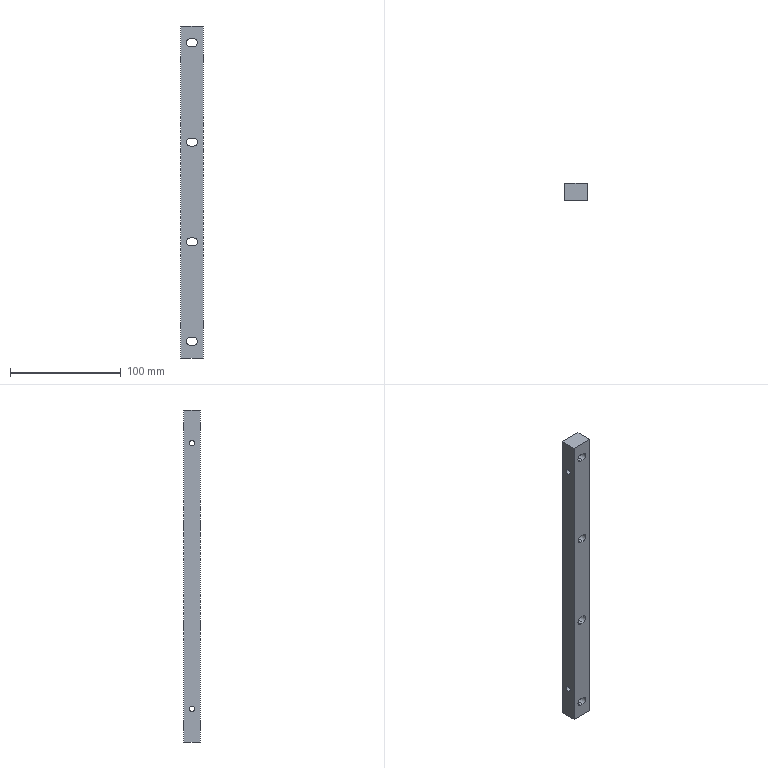Part | NX | 1 solid | 34 faces | box 20 x 15 x 300 mm | volume 85636 mm3 | cylinder 16 | plane 14 | cone 4 | commonest cylinder face diameters 7 x12 5 x4
STEP:
#1=CARTESIAN_POINT('',(263.6,-113.5,-473.5));
#2=VERTEX_POINT('',#1);
#3=CARTESIAN_POINT('',(283.6,-113.5,-473.5));
#4=VERTEX_POINT('',#3);
#5=CARTESIAN_POINT('',(237.204,-113.5,-473.5));
#6=DIRECTION('',(1.,0.,0.));
#7=VECTOR('',#6,1000.);
#8=LINE('',#5,#7);
#9=EDGE_CURVE('',#2,#4,#8,.T.);
#10=ORIENTED_EDGE('',*,*,#9,.F.);
#11=CARTESIAN_POINT('',(263.6,-98.5,-473.5));
#12=VERTEX_POINT('',#11);
#13=CARTESIAN_POINT('',(263.6,-112.5,-473.5));
#14=DIRECTION('',(0.,1.,0.));
#15=VECTOR('',#14,1000.);
#16=LINE('',#13,#15);
#17=EDGE_CURVE('',#2,#12,#16,.T.);
#18=ORIENTED_EDGE('',*,*,#17,.T.);
#19=CARTESIAN_POINT('',(283.6,-98.5,-473.5));
#20=VERTEX_POINT('',#19);
#21=CARTESIAN_POINT('',(237.204,-98.5,-473.5));
#22=DIRECTION('',(-1.,0.,0.));
#23=VECTOR('',#22,1000.);
#24=LINE('',#21,#23);
#25=EDGE_CURVE('',#20,#12,#24,.T.);
#26=ORIENTED_EDGE('',*,*,#25,.F.);
#27=CARTESIAN_POINT('',(283.6,-112.5,-473.5));
#28=DIRECTION('',(0.,-1.,0.));
#29=VECTOR('',#28,1000.);
#30=LINE('',#27,#29);
#31=EDGE_CURVE('',#20,#4,#30,.T.);
#32=ORIENTED_EDGE('',*,*,#31,.T.);
#33=EDGE_LOOP('',(#10,#18,#26,#32));
#34=FACE_BOUND('',#33,.T.);
#35=CARTESIAN_POINT('',(263.6,-112.5,-473.5));
#36=DIRECTION('',(0.,0.,-1.));
#37=DIRECTION('',(0.,-1.,0.));
#38=AXIS2_PLACEMENT_3D('',#35,#36,#37);
#39=PLANE('',#38);
#40=ADVANCED_FACE('',(#34),#39,.T.);
#41=CARTESIAN_POINT('',(263.6,-113.5,-173.5));
#42=VERTEX_POINT('',#41);
#43=CARTESIAN_POINT('',(263.6,-113.5,-531.056));
#44=DIRECTION('',(0.,0.,1.));
#45=VECTOR('',#44,1000.);
#46=LINE('',#43,#45);
#47=EDGE_CURVE('',#2,#42,#46,.T.);
#48=ORIENTED_EDGE('',*,*,#47,.T.);
#49=CARTESIAN_POINT('',(263.6,-98.5,-173.5));
#50=VERTEX_POINT('',#49);
#51=CARTESIAN_POINT('',(263.6,-112.5,-173.5));
#52=DIRECTION('',(0.,-1.,0.));
#53=VECTOR('',#52,1000.);
#54=LINE('',#51,#53);
#55=EDGE_CURVE('',#50,#42,#54,.T.);
#56=ORIENTED_EDGE('',*,*,#55,.F.);
#57=CARTESIAN_POINT('',(263.6,-98.5,-531.056));
#58=DIRECTION('',(0.,0.,1.));
#59=VECTOR('',#58,1000.);
#60=LINE('',#57,#59);
#61=EDGE_CURVE('',#12,#50,#60,.T.);
#62=ORIENTED_EDGE('',*,*,#61,.F.);
#63=ORIENTED_EDGE('',*,*,#17,.F.);
#64=EDGE_LOOP('',(#48,#56,#62,#63));
#65=FACE_BOUND('',#64,.T.);
#66=CARTESIAN_POINT('',(263.6,-106.,-201.));
#67=VERTEX_POINT('',#66);
#68=CARTESIAN_POINT('',(263.6,-106.,-206.));
#69=VERTEX_POINT('',#68);
#70=CARTESIAN_POINT('',(263.6,-106.,-203.5));
#71=DIRECTION('',(1.,0.,0.));
#72=DIRECTION('',(0.,0.,1.));
#73=AXIS2_PLACEMENT_3D('',#70,#71,#72);
#74=CIRCLE('',#73,2.5);
#75=EDGE_CURVE('',#67,#69,#74,.T.);
#76=ORIENTED_EDGE('',*,*,#75,.T.);
#77=CARTESIAN_POINT('',(263.6,-106.,-203.5));
#78=DIRECTION('',(1.,0.,0.));
#79=DIRECTION('',(0.,0.,1.));
#80=AXIS2_PLACEMENT_3D('',#77,#78,#79);
#81=CIRCLE('',#80,2.5);
#82=EDGE_CURVE('',#69,#67,#81,.T.);
#83=ORIENTED_EDGE('',*,*,#82,.T.);
#84=EDGE_LOOP('',(#76,#83));
#85=FACE_BOUND('',#84,.T.);
#86=CARTESIAN_POINT('',(263.6,-106.,-446.));
#87=VERTEX_POINT('',#86);
#88=CARTESIAN_POINT('',(263.6,-106.,-441.));
#89=VERTEX_POINT('',#88);
#90=CARTESIAN_POINT('',(263.6,-106.,-443.5));
#91=DIRECTION('',(1.,0.,0.));
#92=DIRECTION('',(0.,0.,1.));
#93=AXIS2_PLACEMENT_3D('',#90,#91,#92);
#94=CIRCLE('',#93,2.5);
#95=EDGE_CURVE('',#87,#89,#94,.T.);
#96=ORIENTED_EDGE('',*,*,#95,.T.);
#97=CARTESIAN_POINT('',(263.6,-106.,-443.5));
#98=DIRECTION('',(1.,0.,0.));
#99=DIRECTION('',(0.,0.,1.));
#100=AXIS2_PLACEMENT_3D('',#97,#98,#99);
#101=CIRCLE('',#100,2.5);
#102=EDGE_CURVE('',#89,#87,#101,.T.);
#103=ORIENTED_EDGE('',*,*,#102,.T.);
#104=EDGE_LOOP('',(#96,#103));
#105=FACE_BOUND('',#104,.T.);
#106=CARTESIAN_POINT('',(263.6,-112.5,-173.5));
#107=DIRECTION('',(-1.,0.,0.));
#108=DIRECTION('',(0.,0.,1.));
#109=AXIS2_PLACEMENT_3D('',#106,#107,#108);
#110=PLANE('',#109);
#111=ADVANCED_FACE('',(#65,#85,#105),#110,.T.);
#112=CARTESIAN_POINT('',(283.6,-113.5,-173.5));
#113=VERTEX_POINT('',#112);
#114=CARTESIAN_POINT('',(237.204,-113.5,-173.5));
#115=DIRECTION('',(-1.,0.,0.));
#116=VECTOR('',#115,1000.);
#117=LINE('',#114,#116);
#118=EDGE_CURVE('',#113,#42,#117,.T.);
#119=ORIENTED_EDGE('',*,*,#118,.F.);
#120=CARTESIAN_POINT('',(283.6,-98.5,-173.5));
#121=VERTEX_POINT('',#120);
#122=CARTESIAN_POINT('',(283.6,-112.5,-173.5));
#123=DIRECTION('',(0.,1.,0.));
#124=VECTOR('',#123,1000.);
#125=LINE('',#122,#124);
#126=EDGE_CURVE('',#113,#121,#125,.T.);
#127=ORIENTED_EDGE('',*,*,#126,.T.);
#128=CARTESIAN_POINT('',(237.204,-98.5,-173.5));
#129=DIRECTION('',(1.,0.,0.));
#130=VECTOR('',#129,1000.);
#131=LINE('',#128,#130);
#132=EDGE_CURVE('',#50,#121,#131,.T.);
#133=ORIENTED_EDGE('',*,*,#132,.F.);
#134=ORIENTED_EDGE('',*,*,#55,.T.);
#135=EDGE_LOOP('',(#119,#127,#133,#134));
#136=FACE_BOUND('',#135,.T.);
#137=CARTESIAN_POINT('',(278.6,-112.5,-173.5));
#138=DIRECTION('',(0.,0.,1.));
#139=DIRECTION('',(1.,0.,0.));
#140=AXIS2_PLACEMENT_3D('',#137,#138,#139);
#141=PLANE('',#140);
#142=ADVANCED_FACE('',(#136),#141,.T.);
#143=CARTESIAN_POINT('',(283.6,-113.5,-531.056));
#144=DIRECTION('',(0.,0.,-1.));
#145=VECTOR('',#144,1000.);
#146=LINE('',#143,#145);
#147=EDGE_CURVE('',#113,#4,#146,.T.);
#148=ORIENTED_EDGE('',*,*,#147,.T.);
#149=ORIENTED_EDGE('',*,*,#31,.F.);
#150=CARTESIAN_POINT('',(283.6,-98.5,-531.056));
#151=DIRECTION('',(0.,0.,-1.));
#152=VECTOR('',#151,1000.);
#153=LINE('',#150,#152);
#154=EDGE_CURVE('',#121,#20,#153,.T.);
#155=ORIENTED_EDGE('',*,*,#154,.F.);
#156=ORIENTED_EDGE('',*,*,#126,.F.);
#157=EDGE_LOOP('',(#148,#149,#155,#156));
#158=FACE_BOUND('',#157,.T.);
#159=CARTESIAN_POINT('',(283.6,-109.45,-203.5));
#160=VERTEX_POINT('',#159);
#161=CARTESIAN_POINT('',(283.6,-102.55,-203.5));
#162=VERTEX_POINT('',#161);
#163=CARTESIAN_POINT('',(283.6,-106.,-203.5));
#164=DIRECTION('',(1.,0.,0.));
#165=DIRECTION('',(0.,0.,1.));
#166=AXIS2_PLACEMENT_3D('',#163,#164,#165);
#167=CIRCLE('',#166,3.45);
#168=EDGE_CURVE('',#160,#162,#167,.T.);
#169=ORIENTED_EDGE('',*,*,#168,.F.);
#170=CARTESIAN_POINT('',(283.6,-106.,-203.5));
#171=DIRECTION('',(1.,0.,0.));
#172=DIRECTION('',(0.,0.,1.));
#173=AXIS2_PLACEMENT_3D('',#170,#171,#172);
#174=CIRCLE('',#173,3.45);
#175=EDGE_CURVE('',#162,#160,#174,.T.);
#176=ORIENTED_EDGE('',*,*,#175,.F.);
#177=EDGE_LOOP('',(#169,#176));
#178=FACE_BOUND('',#177,.T.);
#179=CARTESIAN_POINT('',(283.6,-109.45,-443.5));
#180=VERTEX_POINT('',#179);
#181=CARTESIAN_POINT('',(283.6,-102.55,-443.5));
#182=VERTEX_POINT('',#181);
#183=CARTESIAN_POINT('',(283.6,-106.,-443.5));
#184=DIRECTION('',(1.,0.,0.));
#185=DIRECTION('',(0.,0.,1.));
#186=AXIS2_PLACEMENT_3D('',#183,#184,#185);
#187=CIRCLE('',#186,3.45);
#188=EDGE_CURVE('',#180,#182,#187,.T.);
#189=ORIENTED_EDGE('',*,*,#188,.F.);
#190=CARTESIAN_POINT('',(283.6,-106.,-443.5));
#191=DIRECTION('',(1.,0.,0.));
#192=DIRECTION('',(0.,0.,1.));
#193=AXIS2_PLACEMENT_3D('',#190,#191,#192);
#194=CIRCLE('',#193,3.45);
#195=EDGE_CURVE('',#182,#180,#194,.T.);
#196=ORIENTED_EDGE('',*,*,#195,.F.);
#197=EDGE_LOOP('',(#189,#196));
#198=FACE_BOUND('',#197,.T.);
#199=CARTESIAN_POINT('',(283.6,-112.5,-473.5));
#200=DIRECTION('',(1.,0.,0.));
#201=DIRECTION('',(0.,1.,0.));
#202=AXIS2_PLACEMENT_3D('',#199,#200,#201);
#203=PLANE('',#202);
#204=ADVANCED_FACE('',(#158,#178,#198),#203,.T.);
#205=CARTESIAN_POINT('',(283.052,-108.5,-203.5));
#206=VERTEX_POINT('',#205);
#207=CARTESIAN_POINT('',(283.052,-106.,-206.));
#208=VERTEX_POINT('',#207);
#209=CARTESIAN_POINT('',(283.052,-106.,-203.5));
#210=DIRECTION('',(1.,0.,0.));
#211=DIRECTION('',(0.,0.,1.));
#212=AXIS2_PLACEMENT_3D('',#209,#210,#211);
#213=CIRCLE('',#212,2.5);
#214=EDGE_CURVE('',#206,#208,#213,.T.);
#215=ORIENTED_EDGE('',*,*,#214,.T.);
#216=CARTESIAN_POINT('',(283.6,-106.,-206.));
#217=DIRECTION('',(1.,0.,0.));
#218=VECTOR('',#217,1000.);
#219=LINE('',#216,#218);
#220=EDGE_CURVE('',#208,#69,#219,.F.);
#221=ORIENTED_EDGE('',*,*,#220,.T.);
#222=ORIENTED_EDGE('',*,*,#75,.F.);
#223=CARTESIAN_POINT('',(283.052,-106.,-201.));
#224=VERTEX_POINT('',#223);
#225=CARTESIAN_POINT('',(283.6,-106.,-201.));
#226=DIRECTION('',(1.,0.,0.));
#227=VECTOR('',#226,1000.);
#228=LINE('',#225,#227);
#229=EDGE_CURVE('',#224,#67,#228,.F.);
#230=ORIENTED_EDGE('',*,*,#229,.F.);
#231=CARTESIAN_POINT('',(283.052,-106.,-203.5));
#232=DIRECTION('',(1.,0.,0.));
#233=DIRECTION('',(0.,0.,1.));
#234=AXIS2_PLACEMENT_3D('',#231,#232,#233);
#235=CIRCLE('',#234,2.5);
#236=EDGE_CURVE('',#224,#206,#235,.T.);
#237=ORIENTED_EDGE('',*,*,#236,.T.);
#238=EDGE_LOOP('',(#215,#221,#222,#230,#237));
#239=FACE_BOUND('',#238,.T.);
#240=CARTESIAN_POINT('',(283.6,-106.,-203.5));
#241=DIRECTION('',(1.,0.,0.));
#242=DIRECTION('',(0.,0.,1.));
#243=AXIS2_PLACEMENT_3D('',#240,#241,#242);
#244=CYLINDRICAL_SURFACE('',#243,2.5);
#245=ADVANCED_FACE('',(#239),#244,.F.);
#246=ORIENTED_EDGE('',*,*,#95,.F.);
#247=CARTESIAN_POINT('',(283.052,-106.,-446.));
#248=VERTEX_POINT('',#247);
#249=CARTESIAN_POINT('',(283.6,-106.,-446.));
#250=DIRECTION('',(1.,0.,0.));
#251=VECTOR('',#250,1000.);
#252=LINE('',#249,#251);
#253=EDGE_CURVE('',#248,#87,#252,.F.);
#254=ORIENTED_EDGE('',*,*,#253,.F.);
#255=CARTESIAN_POINT('',(283.052,-103.5,-443.5));
#256=VERTEX_POINT('',#255);
#257=CARTESIAN_POINT('',(283.052,-106.,-443.5));
#258=DIRECTION('',(1.,0.,0.));
#259=DIRECTION('',(0.,0.,1.));
#260=AXIS2_PLACEMENT_3D('',#257,#258,#259);
#261=CIRCLE('',#260,2.5);
#262=EDGE_CURVE('',#248,#256,#261,.T.);
#263=ORIENTED_EDGE('',*,*,#262,.T.);
#264=CARTESIAN_POINT('',(283.052,-106.,-441.));
#265=VERTEX_POINT('',#264);
#266=CARTESIAN_POINT('',(283.052,-106.,-443.5));
#267=DIRECTION('',(1.,0.,0.));
#268=DIRECTION('',(0.,0.,1.));
#269=AXIS2_PLACEMENT_3D('',#266,#267,#268);
#270=CIRCLE('',#269,2.5);
#271=EDGE_CURVE('',#256,#265,#270,.T.);
#272=ORIENTED_EDGE('',*,*,#271,.T.);
#273=CARTESIAN_POINT('',(283.6,-106.,-441.));
#274=DIRECTION('',(1.,0.,0.));
#275=VECTOR('',#274,1000.);
#276=LINE('',#273,#275);
#277=EDGE_CURVE('',#265,#89,#276,.F.);
#278=ORIENTED_EDGE('',*,*,#277,.T.);
#279=EDGE_LOOP('',(#246,#254,#263,#272,#278));
#280=FACE_BOUND('',#279,.T.);
#281=CARTESIAN_POINT('',(283.6,-106.,-443.5));
#282=DIRECTION('',(1.,0.,0.));
#283=DIRECTION('',(0.,0.,1.));
#284=AXIS2_PLACEMENT_3D('',#281,#282,#283);
#285=CYLINDRICAL_SURFACE('',#284,2.5);
#286=ADVANCED_FACE('',(#280),#285,.F.);
#287=ORIENTED_EDGE('',*,*,#188,.T.);
#288=CARTESIAN_POINT('',(283.052,-103.5,-443.5));
#289=DIRECTION('',(0.5,0.866,0.));
#290=VECTOR('',#289,1000.);
#291=LINE('',#288,#290);
#292=EDGE_CURVE('',#256,#182,#291,.T.);
#293=ORIENTED_EDGE('',*,*,#292,.F.);
#294=ORIENTED_EDGE('',*,*,#262,.F.);
#295=CARTESIAN_POINT('',(283.052,-108.5,-443.5));
#296=VERTEX_POINT('',#295);
#297=CARTESIAN_POINT('',(283.052,-106.,-443.5));
#298=DIRECTION('',(1.,0.,0.));
#299=DIRECTION('',(0.,0.,1.));
#300=AXIS2_PLACEMENT_3D('',#297,#298,#299);
#301=CIRCLE('',#300,2.5);
#302=EDGE_CURVE('',#296,#248,#301,.T.);
#303=ORIENTED_EDGE('',*,*,#302,.F.);
#304=CARTESIAN_POINT('',(283.052,-108.5,-443.5));
#305=DIRECTION('',(0.5,-0.866,0.));
#306=VECTOR('',#305,1000.);
#307=LINE('',#304,#306);
#308=EDGE_CURVE('',#296,#180,#307,.T.);
#309=ORIENTED_EDGE('',*,*,#308,.T.);
#310=EDGE_LOOP('',(#287,#293,#294,#303,#309));
#311=FACE_BOUND('',#310,.T.);
#312=CARTESIAN_POINT('',(283.052,-106.,-443.5));
#313=DIRECTION('',(1.,0.,0.));
#314=DIRECTION('',(0.,-1.,0.));
#315=AXIS2_PLACEMENT_3D('',#312,#313,#314);
#316=CONICAL_SURFACE('',#315,2.5,1.047);
#317=ADVANCED_FACE('',(#311),#316,.F.);
#318=ORIENTED_EDGE('',*,*,#214,.F.);
#319=CARTESIAN_POINT('',(283.052,-108.5,-203.5));
#320=DIRECTION('',(0.5,-0.866,0.));
#321=VECTOR('',#320,1000.);
#322=LINE('',#319,#321);
#323=EDGE_CURVE('',#206,#160,#322,.T.);
#324=ORIENTED_EDGE('',*,*,#323,.T.);
#325=ORIENTED_EDGE('',*,*,#168,.T.);
#326=CARTESIAN_POINT('',(283.052,-103.5,-203.5));
#327=VERTEX_POINT('',#326);
#328=CARTESIAN_POINT('',(283.052,-103.5,-203.5));
#329=DIRECTION('',(0.5,0.866,0.));
#330=VECTOR('',#329,1000.);
#331=LINE('',#328,#330);
#332=EDGE_CURVE('',#327,#162,#331,.T.);
#333=ORIENTED_EDGE('',*,*,#332,.F.);
#334=CARTESIAN_POINT('',(283.052,-106.,-203.5));
#335=DIRECTION('',(1.,0.,0.));
#336=DIRECTION('',(0.,0.,1.));
#337=AXIS2_PLACEMENT_3D('',#334,#335,#336);
#338=CIRCLE('',#337,2.5);
#339=EDGE_CURVE('',#208,#327,#338,.T.);
#340=ORIENTED_EDGE('',*,*,#339,.F.);
#341=EDGE_LOOP('',(#318,#324,#325,#333,#340));
#342=FACE_BOUND('',#341,.T.);
#343=CARTESIAN_POINT('',(283.052,-106.,-203.5));
#344=DIRECTION('',(1.,0.,0.));
#345=DIRECTION('',(0.,-1.,0.));
#346=AXIS2_PLACEMENT_3D('',#343,#344,#345);
#347=CONICAL_SURFACE('',#346,2.5,1.047);
#348=ADVANCED_FACE('',(#342),#347,.F.);
#349=CARTESIAN_POINT('',(275.1,-113.5,-372.));
#350=VERTEX_POINT('',#349);
#351=CARTESIAN_POINT('',(272.1,-113.5,-372.));
#352=VERTEX_POINT('',#351);
#353=CARTESIAN_POINT('',(237.204,-113.5,-372.));
#354=DIRECTION('',(-1.,0.,0.));
#355=VECTOR('',#354,1000.);
#356=LINE('',#353,#355);
#357=EDGE_CURVE('',#350,#352,#356,.T.);
#358=ORIENTED_EDGE('',*,*,#357,.F.);
#359=CARTESIAN_POINT('',(275.1,-98.5,-372.));
#360=VERTEX_POINT('',#359);
#361=CARTESIAN_POINT('',(275.1,-115.,-372.));
#362=DIRECTION('',(0.,1.,0.));
#363=VECTOR('',#362,1000.);
#364=LINE('',#361,#363);
#365=EDGE_CURVE('',#350,#360,#364,.T.);
#366=ORIENTED_EDGE('',*,*,#365,.T.);
#367=CARTESIAN_POINT('',(272.1,-98.5,-372.));
#368=VERTEX_POINT('',#367);
#369=CARTESIAN_POINT('',(237.204,-98.5,-372.));
#370=DIRECTION('',(-1.,0.,0.));
#371=VECTOR('',#370,1000.);
#372=LINE('',#369,#371);
#373=EDGE_CURVE('',#360,#368,#372,.T.);
#374=ORIENTED_EDGE('',*,*,#373,.T.);
#375=CARTESIAN_POINT('',(272.1,-114.,-372.));
#376=DIRECTION('',(0.,1.,0.));
#377=VECTOR('',#376,1000.);
#378=LINE('',#375,#377);
#379=EDGE_CURVE('',#352,#368,#378,.T.);
#380=ORIENTED_EDGE('',*,*,#379,.F.);
#381=EDGE_LOOP('',(#358,#366,#374,#380));
#382=FACE_BOUND('',#381,.T.);
#383=CARTESIAN_POINT('',(272.1,-115.,-372.));
#384=DIRECTION('',(0.,0.,-1.));
#385=DIRECTION('',(0.,-1.,0.));
#386=AXIS2_PLACEMENT_3D('',#383,#384,#385);
#387=PLANE('',#386);
#388=ADVANCED_FACE('',(#382),#387,.F.);
#389=ORIENTED_EDGE('',*,*,#47,.F.);
#390=ORIENTED_EDGE('',*,*,#9,.T.);
#391=ORIENTED_EDGE('',*,*,#147,.F.);
#392=ORIENTED_EDGE('',*,*,#118,.T.);
#393=EDGE_LOOP('',(#389,#390,#391,#392));
#394=FACE_BOUND('',#393,.T.);
#395=CARTESIAN_POINT('',(272.1,-113.5,-365.));
#396=VERTEX_POINT('',#395);
#397=CARTESIAN_POINT('',(275.1,-113.5,-365.));
#398=VERTEX_POINT('',#397);
#399=CARTESIAN_POINT('',(237.204,-113.5,-365.));
#400=DIRECTION('',(1.,0.,0.));
#401=VECTOR('',#400,1000.);
#402=LINE('',#399,#401);
#403=EDGE_CURVE('',#396,#398,#402,.T.);
#404=ORIENTED_EDGE('',*,*,#403,.T.);
#405=CARTESIAN_POINT('',(275.1,-113.5,-368.5));
#406=DIRECTION('',(0.,1.,0.));
#407=DIRECTION('',(-1.,0.,0.));
#408=AXIS2_PLACEMENT_3D('',#405,#406,#407);
#409=CIRCLE('',#408,3.5);
#410=EDGE_CURVE('',#398,#350,#409,.T.);
#411=ORIENTED_EDGE('',*,*,#410,.T.);
#412=ORIENTED_EDGE('',*,*,#357,.T.);
#413=CARTESIAN_POINT('',(268.6,-113.5,-368.5));
#414=VERTEX_POINT('',#413);
#415=CARTESIAN_POINT('',(272.1,-113.5,-368.5));
#416=DIRECTION('',(0.,1.,0.));
#417=DIRECTION('',(-1.,0.,0.));
#418=AXIS2_PLACEMENT_3D('',#415,#416,#417);
#419=CIRCLE('',#418,3.5);
#420=EDGE_CURVE('',#352,#414,#419,.T.);
#421=ORIENTED_EDGE('',*,*,#420,.T.);
#422=CARTESIAN_POINT('',(272.1,-113.5,-368.5));
#423=DIRECTION('',(0.,1.,0.));
#424=DIRECTION('',(-1.,0.,0.));
#425=AXIS2_PLACEMENT_3D('',#422,#423,#424);
#426=CIRCLE('',#425,3.5);
#427=EDGE_CURVE('',#414,#396,#426,.T.);
#428=ORIENTED_EDGE('',*,*,#427,.T.);
#429=EDGE_LOOP('',(#404,#411,#412,#421,#428));
#430=FACE_BOUND('',#429,.T.);
#431=CARTESIAN_POINT('',(272.1,-113.5,-185.));
#432=VERTEX_POINT('',#431);
#433=CARTESIAN_POINT('',(275.1,-113.5,-185.));
#434=VERTEX_POINT('',#433);
#435=CARTESIAN_POINT('',(237.204,-113.5,-185.));
#436=DIRECTION('',(1.,0.,0.));
#437=VECTOR('',#436,1000.);
#438=LINE('',#435,#437);
#439=EDGE_CURVE('',#432,#434,#438,.T.);
#440=ORIENTED_EDGE('',*,*,#439,.T.);
#441=CARTESIAN_POINT('',(275.1,-113.5,-192.));
#442=VERTEX_POINT('',#441);
#443=CARTESIAN_POINT('',(275.1,-113.5,-188.5));
#444=DIRECTION('',(0.,1.,0.));
#445=DIRECTION('',(-1.,0.,0.));
#446=AXIS2_PLACEMENT_3D('',#443,#444,#445);
#447=CIRCLE('',#446,3.5);
#448=EDGE_CURVE('',#434,#442,#447,.T.);
#449=ORIENTED_EDGE('',*,*,#448,.T.);
#450=CARTESIAN_POINT('',(272.1,-113.5,-192.));
#451=VERTEX_POINT('',#450);
#452=CARTESIAN_POINT('',(237.204,-113.5,-192.));
#453=DIRECTION('',(-1.,0.,0.));
#454=VECTOR('',#453,1000.);
#455=LINE('',#452,#454);
#456=EDGE_CURVE('',#442,#451,#455,.T.);
#457=ORIENTED_EDGE('',*,*,#456,.T.);
#458=CARTESIAN_POINT('',(268.6,-113.5,-188.5));
#459=VERTEX_POINT('',#458);
#460=CARTESIAN_POINT('',(272.1,-113.5,-188.5));
#461=DIRECTION('',(0.,1.,0.));
#462=DIRECTION('',(-1.,0.,0.));
#463=AXIS2_PLACEMENT_3D('',#460,#461,#462);
#464=CIRCLE('',#463,3.5);
#465=EDGE_CURVE('',#451,#459,#464,.T.);
#466=ORIENTED_EDGE('',*,*,#465,.T.);
#467=CARTESIAN_POINT('',(272.1,-113.5,-188.5));
#468=DIRECTION('',(0.,1.,0.));
#469=DIRECTION('',(-1.,0.,0.));
#470=AXIS2_PLACEMENT_3D('',#467,#468,#469);
#471=CIRCLE('',#470,3.5);
#472=EDGE_CURVE('',#459,#432,#471,.T.);
#473=ORIENTED_EDGE('',*,*,#472,.T.);
#474=EDGE_LOOP('',(#440,#449,#457,#466,#473));
#475=FACE_BOUND('',#474,.T.);
#476=CARTESIAN_POINT('',(272.1,-113.5,-455.));
#477=VERTEX_POINT('',#476);
#478=CARTESIAN_POINT('',(275.1,-113.5,-455.));
#479=VERTEX_POINT('',#478);
#480=CARTESIAN_POINT('',(237.204,-113.5,-455.));
#481=DIRECTION('',(1.,0.,0.));
#482=VECTOR('',#481,1000.);
#483=LINE('',#480,#482);
#484=EDGE_CURVE('',#477,#479,#483,.T.);
#485=ORIENTED_EDGE('',*,*,#484,.T.);
#486=CARTESIAN_POINT('',(275.1,-113.5,-462.));
#487=VERTEX_POINT('',#486);
#488=CARTESIAN_POINT('',(275.1,-113.5,-458.5));
#489=DIRECTION('',(0.,1.,0.));
#490=DIRECTION('',(-1.,0.,0.));
#491=AXIS2_PLACEMENT_3D('',#488,#489,#490);
#492=CIRCLE('',#491,3.5);
#493=EDGE_CURVE('',#479,#487,#492,.T.);
#494=ORIENTED_EDGE('',*,*,#493,.T.);
#495=CARTESIAN_POINT('',(272.1,-113.5,-462.));
#496=VERTEX_POINT('',#495);
#497=CARTESIAN_POINT('',(237.204,-113.5,-462.));
#498=DIRECTION('',(-1.,0.,0.));
#499=VECTOR('',#498,1000.);
#500=LINE('',#497,#499);
#501=EDGE_CURVE('',#487,#496,#500,.T.);
#502=ORIENTED_EDGE('',*,*,#501,.T.);
#503=CARTESIAN_POINT('',(268.6,-113.5,-458.5));
#504=VERTEX_POINT('',#503);
#505=CARTESIAN_POINT('',(272.1,-113.5,-458.5));
#506=DIRECTION('',(0.,1.,0.));
#507=DIRECTION('',(-1.,0.,0.));
#508=AXIS2_PLACEMENT_3D('',#505,#506,#507);
#509=CIRCLE('',#508,3.5);
#510=EDGE_CURVE('',#496,#504,#509,.T.);
#511=ORIENTED_EDGE('',*,*,#510,.T.);
#512=CARTESIAN_POINT('',(272.1,-113.5,-458.5));
#513=DIRECTION('',(0.,1.,0.));
#514=DIRECTION('',(-1.,0.,0.));
#515=AXIS2_PLACEMENT_3D('',#512,#513,#514);
#516=CIRCLE('',#515,3.5);
#517=EDGE_CURVE('',#504,#477,#516,.T.);
#518=ORIENTED_EDGE('',*,*,#517,.T.);
#519=EDGE_LOOP('',(#485,#494,#502,#511,#518));
#520=FACE_BOUND('',#519,.T.);
#521=CARTESIAN_POINT('',(272.1,-113.5,-275.));
#522=VERTEX_POINT('',#521);
#523=CARTESIAN_POINT('',(275.1,-113.5,-275.));
#524=VERTEX_POINT('',#523);
#525=CARTESIAN_POINT('',(237.204,-113.5,-275.));
#526=DIRECTION('',(1.,0.,0.));
#527=VECTOR('',#526,1000.);
#528=LINE('',#525,#527);
#529=EDGE_CURVE('',#522,#524,#528,.T.);
#530=ORIENTED_EDGE('',*,*,#529,.T.);
#531=CARTESIAN_POINT('',(275.1,-113.5,-282.));
#532=VERTEX_POINT('',#531);
#533=CARTESIAN_POINT('',(275.1,-113.5,-278.5));
#534=DIRECTION('',(0.,1.,0.));
#535=DIRECTION('',(-1.,0.,0.));
#536=AXIS2_PLACEMENT_3D('',#533,#534,#535);
#537=CIRCLE('',#536,3.5);
#538=EDGE_CURVE('',#524,#532,#537,.T.);
#539=ORIENTED_EDGE('',*,*,#538,.T.);
#540=CARTESIAN_POINT('',(272.1,-113.5,-282.));
#541=VERTEX_POINT('',#540);
#542=CARTESIAN_POINT('',(237.204,-113.5,-282.));
#543=DIRECTION('',(-1.,0.,0.));
#544=VECTOR('',#543,1000.);
#545=LINE('',#542,#544);
#546=EDGE_CURVE('',#532,#541,#545,.T.);
#547=ORIENTED_EDGE('',*,*,#546,.T.);
#548=CARTESIAN_POINT('',(268.6,-113.5,-278.5));
#549=VERTEX_POINT('',#548);
#550=CARTESIAN_POINT('',(272.1,-113.5,-278.5));
#551=DIRECTION('',(0.,1.,0.));
#552=DIRECTION('',(-1.,0.,0.));
#553=AXIS2_PLACEMENT_3D('',#550,#551,#552);
#554=CIRCLE('',#553,3.5);
#555=EDGE_CURVE('',#541,#549,#554,.T.);
#556=ORIENTED_EDGE('',*,*,#555,.T.);
#557=CARTESIAN_POINT('',(272.1,-113.5,-278.5));
#558=DIRECTION('',(0.,1.,0.));
#559=DIRECTION('',(-1.,0.,0.));
#560=AXIS2_PLACEMENT_3D('',#557,#558,#559);
#561=CIRCLE('',#560,3.5);
#562=EDGE_CURVE('',#549,#522,#561,.T.);
#563=ORIENTED_EDGE('',*,*,#562,.T.);
#564=EDGE_LOOP('',(#530,#539,#547,#556,#563));
#565=FACE_BOUND('',#564,.T.);
#566=CARTESIAN_POINT('',(237.204,-113.5,-531.056));
#567=DIRECTION('',(0.,1.,0.));
#568=DIRECTION('',(1.,0.,0.));
#569=AXIS2_PLACEMENT_3D('',#566,#567,#568);
#570=PLANE('',#569);
#571=ADVANCED_FACE('',(#394,#430,#475,#520,#565),#570,.F.);
#572=ORIENTED_EDGE('',*,*,#403,.F.);
#573=CARTESIAN_POINT('',(272.1,-98.5,-365.));
#574=VERTEX_POINT('',#573);
#575=CARTESIAN_POINT('',(272.1,-115.,-365.));
#576=DIRECTION('',(0.,1.,0.));
#577=VECTOR('',#576,1000.);
#578=LINE('',#575,#577);
#579=EDGE_CURVE('',#396,#574,#578,.T.);
#580=ORIENTED_EDGE('',*,*,#579,.T.);
#581=CARTESIAN_POINT('',(275.1,-98.5,-365.));
#582=VERTEX_POINT('',#581);
#583=CARTESIAN_POINT('',(237.204,-98.5,-365.));
#584=DIRECTION('',(1.,0.,0.));
#585=VECTOR('',#584,1000.);
#586=LINE('',#583,#585);
#587=EDGE_CURVE('',#574,#582,#586,.T.);
#588=ORIENTED_EDGE('',*,*,#587,.T.);
#589=CARTESIAN_POINT('',(275.1,-115.,-365.));
#590=DIRECTION('',(0.,1.,0.));
#591=VECTOR('',#590,1000.);
#592=LINE('',#589,#591);
#593=EDGE_CURVE('',#398,#582,#592,.T.);
#594=ORIENTED_EDGE('',*,*,#593,.F.);
#595=EDGE_LOOP('',(#572,#580,#588,#594));
#596=FACE_BOUND('',#595,.T.);
#597=CARTESIAN_POINT('',(275.1,-115.,-365.));
#598=DIRECTION('',(0.,0.,1.));
#599=DIRECTION('',(1.,0.,0.));
#600=AXIS2_PLACEMENT_3D('',#597,#598,#599);
#601=PLANE('',#600);
#602=ADVANCED_FACE('',(#596),#601,.F.);
#603=ORIENTED_EDGE('',*,*,#456,.F.);
#604=CARTESIAN_POINT('',(275.1,-98.5,-192.));
#605=VERTEX_POINT('',#604);
#606=CARTESIAN_POINT('',(275.1,-115.,-192.));
#607=DIRECTION('',(0.,1.,0.));
#608=VECTOR('',#607,1000.);
#609=LINE('',#606,#608);
#610=EDGE_CURVE('',#442,#605,#609,.T.);
#611=ORIENTED_EDGE('',*,*,#610,.T.);
#612=CARTESIAN_POINT('',(272.1,-98.5,-192.));
#613=VERTEX_POINT('',#612);
#614=CARTESIAN_POINT('',(237.204,-98.5,-192.));
#615=DIRECTION('',(-1.,0.,0.));
#616=VECTOR('',#615,1000.);
#617=LINE('',#614,#616);
#618=EDGE_CURVE('',#605,#613,#617,.T.);
#619=ORIENTED_EDGE('',*,*,#618,.T.);
#620=CARTESIAN_POINT('',(272.1,-114.,-192.));
#621=DIRECTION('',(0.,1.,0.));
#622=VECTOR('',#621,1000.);
#623=LINE('',#620,#622);
#624=EDGE_CURVE('',#451,#613,#623,.T.);
#625=ORIENTED_EDGE('',*,*,#624,.F.);
#626=EDGE_LOOP('',(#603,#611,#619,#625));
#627=FACE_BOUND('',#626,.T.);
#628=CARTESIAN_POINT('',(272.1,-115.,-192.));
#629=DIRECTION('',(0.,0.,-1.));
#630=DIRECTION('',(0.,-1.,0.));
#631=AXIS2_PLACEMENT_3D('',#628,#629,#630);
#632=PLANE('',#631);
#633=ADVANCED_FACE('',(#627),#632,.F.);
#634=ORIENTED_EDGE('',*,*,#132,.T.);
#635=ORIENTED_EDGE('',*,*,#154,.T.);
#636=ORIENTED_EDGE('',*,*,#25,.T.);
#637=ORIENTED_EDGE('',*,*,#61,.T.);
#638=EDGE_LOOP('',(#634,#635,#636,#637));
#639=FACE_BOUND('',#638,.T.);
#640=CARTESIAN_POINT('',(275.1,-98.5,-462.));
#641=VERTEX_POINT('',#640);
#642=CARTESIAN_POINT('',(272.1,-98.5,-462.));
#643=VERTEX_POINT('',#642);
#644=CARTESIAN_POINT('',(237.204,-98.5,-462.));
#645=DIRECTION('',(-1.,0.,0.));
#646=VECTOR('',#645,1000.);
#647=LINE('',#644,#646);
#648=EDGE_CURVE('',#641,#643,#647,.T.);
#649=ORIENTED_EDGE('',*,*,#648,.F.);
#650=CARTESIAN_POINT('',(275.1,-98.5,-455.));
#651=VERTEX_POINT('',#650);
#652=CARTESIAN_POINT('',(275.1,-98.5,-458.5));
#653=DIRECTION('',(0.,1.,0.));
#654=DIRECTION('',(-1.,0.,0.));
#655=AXIS2_PLACEMENT_3D('',#652,#653,#654);
#656=CIRCLE('',#655,3.5);
#657=EDGE_CURVE('',#651,#641,#656,.T.);
#658=ORIENTED_EDGE('',*,*,#657,.F.);
#659=CARTESIAN_POINT('',(272.1,-98.5,-455.));
#660=VERTEX_POINT('',#659);
#661=CARTESIAN_POINT('',(237.204,-98.5,-455.));
#662=DIRECTION('',(1.,0.,0.));
#663=VECTOR('',#662,1000.);
#664=LINE('',#661,#663);
#665=EDGE_CURVE('',#660,#651,#664,.T.);
#666=ORIENTED_EDGE('',*,*,#665,.F.);
#667=CARTESIAN_POINT('',(268.6,-98.5,-458.5));
#668=VERTEX_POINT('',#667);
#669=CARTESIAN_POINT('',(272.1,-98.5,-458.5));
#670=DIRECTION('',(0.,1.,0.));
#671=DIRECTION('',(-1.,0.,0.));
#672=AXIS2_PLACEMENT_3D('',#669,#670,#671);
#673=CIRCLE('',#672,3.5);
#674=EDGE_CURVE('',#668,#660,#673,.T.);
#675=ORIENTED_EDGE('',*,*,#674,.F.);
#676=CARTESIAN_POINT('',(272.1,-98.5,-458.5));
#677=DIRECTION('',(0.,1.,0.));
#678=DIRECTION('',(-1.,0.,0.));
#679=AXIS2_PLACEMENT_3D('',#676,#677,#678);
#680=CIRCLE('',#679,3.5);
#681=EDGE_CURVE('',#643,#668,#680,.T.);
#682=ORIENTED_EDGE('',*,*,#681,.F.);
#683=EDGE_LOOP('',(#649,#658,#666,#675,#682));
#684=FACE_BOUND('',#683,.T.);
#685=CARTESIAN_POINT('',(272.1,-98.5,-282.));
#686=VERTEX_POINT('',#685);
#687=CARTESIAN_POINT('',(268.6,-98.5,-278.5));
#688=VERTEX_POINT('',#687);
#689=CARTESIAN_POINT('',(272.1,-98.5,-278.5));
#690=DIRECTION('',(0.,1.,0.));
#691=DIRECTION('',(-1.,0.,0.));
#692=AXIS2_PLACEMENT_3D('',#689,#690,#691);
#693=CIRCLE('',#692,3.5);
#694=EDGE_CURVE('',#686,#688,#693,.T.);
#695=ORIENTED_EDGE('',*,*,#694,.F.);
#696=CARTESIAN_POINT('',(275.1,-98.5,-282.));
#697=VERTEX_POINT('',#696);
#698=CARTESIAN_POINT('',(237.204,-98.5,-282.));
#699=DIRECTION('',(-1.,0.,0.));
#700=VECTOR('',#699,1000.);
#701=LINE('',#698,#700);
#702=EDGE_CURVE('',#697,#686,#701,.T.);
#703=ORIENTED_EDGE('',*,*,#702,.F.);
#704=CARTESIAN_POINT('',(275.1,-98.5,-275.));
#705=VERTEX_POINT('',#704);
#706=CARTESIAN_POINT('',(275.1,-98.5,-278.5));
#707=DIRECTION('',(0.,1.,0.));
#708=DIRECTION('',(-1.,0.,0.));
#709=AXIS2_PLACEMENT_3D('',#706,#707,#708);
#710=CIRCLE('',#709,3.5);
#711=EDGE_CURVE('',#705,#697,#710,.T.);
#712=ORIENTED_EDGE('',*,*,#711,.F.);
#713=CARTESIAN_POINT('',(272.1,-98.5,-275.));
#714=VERTEX_POINT('',#713);
#715=CARTESIAN_POINT('',(237.204,-98.5,-275.));
#716=DIRECTION('',(1.,0.,0.));
#717=VECTOR('',#716,1000.);
#718=LINE('',#715,#717);
#719=EDGE_CURVE('',#714,#705,#718,.T.);
#720=ORIENTED_EDGE('',*,*,#719,.F.);
#721=CARTESIAN_POINT('',(272.1,-98.5,-278.5));
#722=DIRECTION('',(0.,1.,0.));
#723=DIRECTION('',(-1.,0.,0.));
#724=AXIS2_PLACEMENT_3D('',#721,#722,#723);
#725=CIRCLE('',#724,3.5);
#726=EDGE_CURVE('',#688,#714,#725,.T.);
#727=ORIENTED_EDGE('',*,*,#726,.F.);
#728=EDGE_LOOP('',(#695,#703,#712,#720,#727));
#729=FACE_BOUND('',#728,.T.);
#730=ORIENTED_EDGE('',*,*,#618,.F.);
#731=CARTESIAN_POINT('',(275.1,-98.5,-185.));
#732=VERTEX_POINT('',#731);
#733=CARTESIAN_POINT('',(275.1,-98.5,-188.5));
#734=DIRECTION('',(0.,1.,0.));
#735=DIRECTION('',(-1.,0.,0.));
#736=AXIS2_PLACEMENT_3D('',#733,#734,#735);
#737=CIRCLE('',#736,3.5);
#738=EDGE_CURVE('',#732,#605,#737,.T.);
#739=ORIENTED_EDGE('',*,*,#738,.F.);
#740=CARTESIAN_POINT('',(272.1,-98.5,-185.));
#741=VERTEX_POINT('',#740);
#742=CARTESIAN_POINT('',(237.204,-98.5,-185.));
#743=DIRECTION('',(1.,0.,0.));
#744=VECTOR('',#743,1000.);
#745=LINE('',#742,#744);
#746=EDGE_CURVE('',#741,#732,#745,.T.);
#747=ORIENTED_EDGE('',*,*,#746,.F.);
#748=CARTESIAN_POINT('',(268.6,-98.5,-188.5));
#749=VERTEX_POINT('',#748);
#750=CARTESIAN_POINT('',(272.1,-98.5,-188.5));
#751=DIRECTION('',(0.,1.,0.));
#752=DIRECTION('',(-1.,0.,0.));
#753=AXIS2_PLACEMENT_3D('',#750,#751,#752);
#754=CIRCLE('',#753,3.5);
#755=EDGE_CURVE('',#749,#741,#754,.T.);
#756=ORIENTED_EDGE('',*,*,#755,.F.);
#757=CARTESIAN_POINT('',(272.1,-98.5,-188.5));
#758=DIRECTION('',(0.,1.,0.));
#759=DIRECTION('',(-1.,0.,0.));
#760=AXIS2_PLACEMENT_3D('',#757,#758,#759);
#761=CIRCLE('',#760,3.5);
#762=EDGE_CURVE('',#613,#749,#761,.T.);
#763=ORIENTED_EDGE('',*,*,#762,.F.);
#764=EDGE_LOOP('',(#730,#739,#747,#756,#763));
#765=FACE_BOUND('',#764,.T.);
#766=CARTESIAN_POINT('',(268.6,-98.5,-368.5));
#767=VERTEX_POINT('',#766);
#768=CARTESIAN_POINT('',(272.1,-98.5,-368.5));
#769=DIRECTION('',(0.,1.,0.));
#770=DIRECTION('',(-1.,0.,0.));
#771=AXIS2_PLACEMENT_3D('',#768,#769,#770);
#772=CIRCLE('',#771,3.5);
#773=EDGE_CURVE('',#368,#767,#772,.T.);
#774=ORIENTED_EDGE('',*,*,#773,.F.);
#775=ORIENTED_EDGE('',*,*,#373,.F.);
#776=CARTESIAN_POINT('',(275.1,-98.5,-368.5));
#777=DIRECTION('',(0.,1.,0.));
#778=DIRECTION('',(-1.,0.,0.));
#779=AXIS2_PLACEMENT_3D('',#776,#777,#778);
#780=CIRCLE('',#779,3.5);
#781=EDGE_CURVE('',#582,#360,#780,.T.);
#782=ORIENTED_EDGE('',*,*,#781,.F.);
#783=ORIENTED_EDGE('',*,*,#587,.F.);
#784=CARTESIAN_POINT('',(272.1,-98.5,-368.5));
#785=DIRECTION('',(0.,1.,0.));
#786=DIRECTION('',(-1.,0.,0.));
#787=AXIS2_PLACEMENT_3D('',#784,#785,#786);
#788=CIRCLE('',#787,3.5);
#789=EDGE_CURVE('',#767,#574,#788,.T.);
#790=ORIENTED_EDGE('',*,*,#789,.F.);
#791=EDGE_LOOP('',(#774,#775,#782,#783,#790));
#792=FACE_BOUND('',#791,.T.);
#793=CARTESIAN_POINT('',(237.204,-98.5,-531.056));
#794=DIRECTION('',(0.,1.,0.));
#795=DIRECTION('',(1.,0.,0.));
#796=AXIS2_PLACEMENT_3D('',#793,#794,#795);
#797=PLANE('',#796);
#798=ADVANCED_FACE('',(#639,#684,#729,#765,#792),#797,.T.);
#799=CARTESIAN_POINT('',(268.6,-115.,-458.5));
#800=DIRECTION('',(0.,1.,0.));
#801=VECTOR('',#800,1000.);
#802=LINE('',#799,#801);
#803=EDGE_CURVE('',#504,#668,#802,.T.);
#804=ORIENTED_EDGE('',*,*,#803,.F.);
#805=ORIENTED_EDGE('',*,*,#510,.F.);
#806=CARTESIAN_POINT('',(272.1,-114.,-462.));
#807=DIRECTION('',(0.,1.,0.));
#808=VECTOR('',#807,1000.);
#809=LINE('',#806,#808);
#810=EDGE_CURVE('',#496,#643,#809,.T.);
#811=ORIENTED_EDGE('',*,*,#810,.T.);
#812=ORIENTED_EDGE('',*,*,#681,.T.);
#813=EDGE_LOOP('',(#804,#805,#811,#812));
#814=FACE_BOUND('',#813,.T.);
#815=CARTESIAN_POINT('',(272.1,-115.,-458.5));
#816=DIRECTION('',(0.,1.,0.));
#817=DIRECTION('',(-1.,0.,0.));
#818=AXIS2_PLACEMENT_3D('',#815,#816,#817);
#819=CYLINDRICAL_SURFACE('',#818,3.5);
#820=ADVANCED_FACE('',(#814),#819,.F.);
#821=CARTESIAN_POINT('',(268.6,-115.,-368.5));
#822=DIRECTION('',(0.,1.,0.));
#823=VECTOR('',#822,1000.);
#824=LINE('',#821,#823);
#825=EDGE_CURVE('',#414,#767,#824,.T.);
#826=ORIENTED_EDGE('',*,*,#825,.F.);
#827=ORIENTED_EDGE('',*,*,#420,.F.);
#828=ORIENTED_EDGE('',*,*,#379,.T.);
#829=ORIENTED_EDGE('',*,*,#773,.T.);
#830=EDGE_LOOP('',(#826,#827,#828,#829));
#831=FACE_BOUND('',#830,.T.);
#832=CARTESIAN_POINT('',(272.1,-115.,-368.5));
#833=DIRECTION('',(0.,1.,0.));
#834=DIRECTION('',(-1.,0.,0.));
#835=AXIS2_PLACEMENT_3D('',#832,#833,#834);
#836=CYLINDRICAL_SURFACE('',#835,3.5);
#837=ADVANCED_FACE('',(#831),#836,.F.);
#838=ORIENTED_EDGE('',*,*,#484,.F.);
#839=CARTESIAN_POINT('',(272.1,-115.,-455.));
#840=DIRECTION('',(0.,1.,0.));
#841=VECTOR('',#840,1000.);
#842=LINE('',#839,#841);
#843=EDGE_CURVE('',#477,#660,#842,.T.);
#844=ORIENTED_EDGE('',*,*,#843,.T.);
#845=ORIENTED_EDGE('',*,*,#665,.T.);
#846=CARTESIAN_POINT('',(275.1,-115.,-455.));
#847=DIRECTION('',(0.,1.,0.));
#848=VECTOR('',#847,1000.);
#849=LINE('',#846,#848);
#850=EDGE_CURVE('',#479,#651,#849,.T.);
#851=ORIENTED_EDGE('',*,*,#850,.F.);
#852=EDGE_LOOP('',(#838,#844,#845,#851));
#853=FACE_BOUND('',#852,.T.);
#854=CARTESIAN_POINT('',(275.1,-115.,-455.));
#855=DIRECTION('',(0.,0.,1.));
#856=DIRECTION('',(1.,0.,0.));
#857=AXIS2_PLACEMENT_3D('',#854,#855,#856);
#858=PLANE('',#857);
#859=ADVANCED_FACE('',(#853),#858,.F.);
#860=ORIENTED_EDGE('',*,*,#746,.T.);
#861=CARTESIAN_POINT('',(275.1,-115.,-185.));
#862=DIRECTION('',(0.,1.,0.));
#863=VECTOR('',#862,1000.);
#864=LINE('',#861,#863);
#865=EDGE_CURVE('',#434,#732,#864,.T.);
#866=ORIENTED_EDGE('',*,*,#865,.F.);
#867=ORIENTED_EDGE('',*,*,#439,.F.);
#868=CARTESIAN_POINT('',(272.1,-115.,-185.));
#869=DIRECTION('',(0.,1.,0.));
#870=VECTOR('',#869,1000.);
#871=LINE('',#868,#870);
#872=EDGE_CURVE('',#432,#741,#871,.T.);
#873=ORIENTED_EDGE('',*,*,#872,.T.);
#874=EDGE_LOOP('',(#860,#866,#867,#873));
#875=FACE_BOUND('',#874,.T.);
#876=CARTESIAN_POINT('',(275.1,-115.,-185.));
#877=DIRECTION('',(0.,0.,1.));
#878=DIRECTION('',(1.,0.,0.));
#879=AXIS2_PLACEMENT_3D('',#876,#877,#878);
#880=PLANE('',#879);
#881=ADVANCED_FACE('',(#875),#880,.F.);
#882=ORIENTED_EDGE('',*,*,#648,.T.);
#883=ORIENTED_EDGE('',*,*,#810,.F.);
#884=ORIENTED_EDGE('',*,*,#501,.F.);
#885=CARTESIAN_POINT('',(275.1,-115.,-462.));
#886=DIRECTION('',(0.,1.,0.));
#887=VECTOR('',#886,1000.);
#888=LINE('',#885,#887);
#889=EDGE_CURVE('',#487,#641,#888,.T.);
#890=ORIENTED_EDGE('',*,*,#889,.T.);
#891=EDGE_LOOP('',(#882,#883,#884,#890));
#892=FACE_BOUND('',#891,.T.);
#893=CARTESIAN_POINT('',(272.1,-115.,-462.));
#894=DIRECTION('',(0.,0.,-1.));
#895=DIRECTION('',(0.,-1.,0.));
#896=AXIS2_PLACEMENT_3D('',#893,#894,#895);
#897=PLANE('',#896);
#898=ADVANCED_FACE('',(#892),#897,.F.);
#899=ORIENTED_EDGE('',*,*,#657,.T.);
#900=ORIENTED_EDGE('',*,*,#889,.F.);
#901=ORIENTED_EDGE('',*,*,#493,.F.);
#902=ORIENTED_EDGE('',*,*,#850,.T.);
#903=EDGE_LOOP('',(#899,#900,#901,#902));
#904=FACE_BOUND('',#903,.T.);
#905=CARTESIAN_POINT('',(275.1,-115.,-458.5));
#906=DIRECTION('',(0.,1.,0.));
#907=DIRECTION('',(-1.,0.,0.));
#908=AXIS2_PLACEMENT_3D('',#905,#906,#907);
#909=CYLINDRICAL_SURFACE('',#908,3.5);
#910=ADVANCED_FACE('',(#904),#909,.F.);
#911=ORIENTED_EDGE('',*,*,#529,.F.);
#912=CARTESIAN_POINT('',(272.1,-114.,-275.));
#913=DIRECTION('',(0.,1.,0.));
#914=VECTOR('',#913,1000.);
#915=LINE('',#912,#914);
#916=EDGE_CURVE('',#522,#714,#915,.T.);
#917=ORIENTED_EDGE('',*,*,#916,.T.);
#918=ORIENTED_EDGE('',*,*,#719,.T.);
#919=CARTESIAN_POINT('',(275.1,-115.,-275.));
#920=DIRECTION('',(0.,1.,0.));
#921=VECTOR('',#920,1000.);
#922=LINE('',#919,#921);
#923=EDGE_CURVE('',#524,#705,#922,.T.);
#924=ORIENTED_EDGE('',*,*,#923,.F.);
#925=EDGE_LOOP('',(#911,#917,#918,#924));
#926=FACE_BOUND('',#925,.T.);
#927=CARTESIAN_POINT('',(275.1,-115.,-275.));
#928=DIRECTION('',(0.,0.,1.));
#929=DIRECTION('',(1.,0.,0.));
#930=AXIS2_PLACEMENT_3D('',#927,#928,#929);
#931=PLANE('',#930);
#932=ADVANCED_FACE('',(#926),#931,.F.);
#933=ORIENTED_EDGE('',*,*,#738,.T.);
#934=ORIENTED_EDGE('',*,*,#610,.F.);
#935=ORIENTED_EDGE('',*,*,#448,.F.);
#936=ORIENTED_EDGE('',*,*,#865,.T.);
#937=EDGE_LOOP('',(#933,#934,#935,#936));
#938=FACE_BOUND('',#937,.T.);
#939=CARTESIAN_POINT('',(275.1,-115.,-188.5));
#940=DIRECTION('',(0.,1.,0.));
#941=DIRECTION('',(-1.,0.,0.));
#942=AXIS2_PLACEMENT_3D('',#939,#940,#941);
#943=CYLINDRICAL_SURFACE('',#942,3.5);
#944=ADVANCED_FACE('',(#938),#943,.F.);
#945=ORIENTED_EDGE('',*,*,#702,.T.);
#946=CARTESIAN_POINT('',(272.1,-114.,-282.));
#947=DIRECTION('',(0.,1.,0.));
#948=VECTOR('',#947,1000.);
#949=LINE('',#946,#948);
#950=EDGE_CURVE('',#541,#686,#949,.T.);
#951=ORIENTED_EDGE('',*,*,#950,.F.);
#952=ORIENTED_EDGE('',*,*,#546,.F.);
#953=CARTESIAN_POINT('',(275.1,-115.,-282.));
#954=DIRECTION('',(0.,1.,0.));
#955=VECTOR('',#954,1000.);
#956=LINE('',#953,#955);
#957=EDGE_CURVE('',#532,#697,#956,.T.);
#958=ORIENTED_EDGE('',*,*,#957,.T.);
#959=EDGE_LOOP('',(#945,#951,#952,#958));
#960=FACE_BOUND('',#959,.T.);
#961=CARTESIAN_POINT('',(272.1,-115.,-282.));
#962=DIRECTION('',(0.,0.,-1.));
#963=DIRECTION('',(0.,-1.,0.));
#964=AXIS2_PLACEMENT_3D('',#961,#962,#963);
#965=PLANE('',#964);
#966=ADVANCED_FACE('',(#960),#965,.F.);
#967=ORIENTED_EDGE('',*,*,#538,.F.);
#968=ORIENTED_EDGE('',*,*,#923,.T.);
#969=ORIENTED_EDGE('',*,*,#711,.T.);
#970=ORIENTED_EDGE('',*,*,#957,.F.);
#971=EDGE_LOOP('',(#967,#968,#969,#970));
#972=FACE_BOUND('',#971,.T.);
#973=CARTESIAN_POINT('',(275.1,-115.,-278.5));
#974=DIRECTION('',(0.,1.,0.));
#975=DIRECTION('',(-1.,0.,0.));
#976=AXIS2_PLACEMENT_3D('',#973,#974,#975);
#977=CYLINDRICAL_SURFACE('',#976,3.5);
#978=ADVANCED_FACE('',(#972),#977,.F.);
#979=ORIENTED_EDGE('',*,*,#410,.F.);
#980=ORIENTED_EDGE('',*,*,#593,.T.);
#981=ORIENTED_EDGE('',*,*,#781,.T.);
#982=ORIENTED_EDGE('',*,*,#365,.F.);
#983=EDGE_LOOP('',(#979,#980,#981,#982));
#984=FACE_BOUND('',#983,.T.);
#985=CARTESIAN_POINT('',(275.1,-115.,-368.5));
#986=DIRECTION('',(0.,1.,0.));
#987=DIRECTION('',(-1.,0.,0.));
#988=AXIS2_PLACEMENT_3D('',#985,#986,#987);
#989=CYLINDRICAL_SURFACE('',#988,3.5);
#990=ADVANCED_FACE('',(#984),#989,.F.);
#991=CARTESIAN_POINT('',(268.6,-115.,-278.5));
#992=DIRECTION('',(0.,1.,0.));
#993=VECTOR('',#992,1000.);
#994=LINE('',#991,#993);
#995=EDGE_CURVE('',#549,#688,#994,.T.);
#996=ORIENTED_EDGE('',*,*,#995,.F.);
#997=ORIENTED_EDGE('',*,*,#555,.F.);
#998=ORIENTED_EDGE('',*,*,#950,.T.);
#999=ORIENTED_EDGE('',*,*,#694,.T.);
#1000=EDGE_LOOP('',(#996,#997,#998,#999));
#1001=FACE_BOUND('',#1000,.T.);
#1002=CARTESIAN_POINT('',(272.1,-115.,-278.5));
#1003=DIRECTION('',(0.,1.,0.));
#1004=DIRECTION('',(-1.,0.,0.));
#1005=AXIS2_PLACEMENT_3D('',#1002,#1003,#1004);
#1006=CYLINDRICAL_SURFACE('',#1005,3.5);
#1007=ADVANCED_FACE('',(#1001),#1006,.F.);
#1008=CARTESIAN_POINT('',(268.6,-115.,-188.5));
#1009=DIRECTION('',(0.,1.,0.));
#1010=VECTOR('',#1009,1000.);
#1011=LINE('',#1008,#1010);
#1012=EDGE_CURVE('',#459,#749,#1011,.T.);
#1013=ORIENTED_EDGE('',*,*,#1012,.F.);
#1014=ORIENTED_EDGE('',*,*,#465,.F.);
#1015=ORIENTED_EDGE('',*,*,#624,.T.);
#1016=ORIENTED_EDGE('',*,*,#762,.T.);
#1017=EDGE_LOOP('',(#1013,#1014,#1015,#1016));
#1018=FACE_BOUND('',#1017,.T.);
#1019=CARTESIAN_POINT('',(272.1,-115.,-188.5));
#1020=DIRECTION('',(0.,1.,0.));
#1021=DIRECTION('',(-1.,0.,0.));
#1022=AXIS2_PLACEMENT_3D('',#1019,#1020,#1021);
#1023=CYLINDRICAL_SURFACE('',#1022,3.5);
#1024=ADVANCED_FACE('',(#1018),#1023,.F.);
#1025=ORIENTED_EDGE('',*,*,#271,.F.);
#1026=ORIENTED_EDGE('',*,*,#292,.T.);
#1027=ORIENTED_EDGE('',*,*,#195,.T.);
#1028=ORIENTED_EDGE('',*,*,#308,.F.);
#1029=CARTESIAN_POINT('',(283.052,-106.,-443.5));
#1030=DIRECTION('',(1.,0.,0.));
#1031=DIRECTION('',(0.,0.,1.));
#1032=AXIS2_PLACEMENT_3D('',#1029,#1030,#1031);
#1033=CIRCLE('',#1032,2.5);
#1034=EDGE_CURVE('',#265,#296,#1033,.T.);
#1035=ORIENTED_EDGE('',*,*,#1034,.F.);
#1036=EDGE_LOOP('',(#1025,#1026,#1027,#1028,#1035));
#1037=FACE_BOUND('',#1036,.T.);
#1038=CARTESIAN_POINT('',(283.052,-106.,-443.5));
#1039=DIRECTION('',(1.,0.,0.));
#1040=DIRECTION('',(0.,-1.,0.));
#1041=AXIS2_PLACEMENT_3D('',#1038,#1039,#1040);
#1042=CONICAL_SURFACE('',#1041,2.5,1.047);
#1043=ADVANCED_FACE('',(#1037),#1042,.F.);
#1044=ORIENTED_EDGE('',*,*,#253,.T.);
#1045=ORIENTED_EDGE('',*,*,#102,.F.);
#1046=ORIENTED_EDGE('',*,*,#277,.F.);
#1047=ORIENTED_EDGE('',*,*,#1034,.T.);
#1048=ORIENTED_EDGE('',*,*,#302,.T.);
#1049=EDGE_LOOP('',(#1044,#1045,#1046,#1047,#1048));
#1050=FACE_BOUND('',#1049,.T.);
#1051=CARTESIAN_POINT('',(283.6,-106.,-443.5));
#1052=DIRECTION('',(1.,0.,0.));
#1053=DIRECTION('',(0.,0.,1.));
#1054=AXIS2_PLACEMENT_3D('',#1051,#1052,#1053);
#1055=CYLINDRICAL_SURFACE('',#1054,2.5);
#1056=ADVANCED_FACE('',(#1050),#1055,.F.);
#1057=ORIENTED_EDGE('',*,*,#220,.F.);
#1058=ORIENTED_EDGE('',*,*,#339,.T.);
#1059=CARTESIAN_POINT('',(283.052,-106.,-203.5));
#1060=DIRECTION('',(1.,0.,0.));
#1061=DIRECTION('',(0.,0.,1.));
#1062=AXIS2_PLACEMENT_3D('',#1059,#1060,#1061);
#1063=CIRCLE('',#1062,2.5);
#1064=EDGE_CURVE('',#327,#224,#1063,.T.);
#1065=ORIENTED_EDGE('',*,*,#1064,.T.);
#1066=ORIENTED_EDGE('',*,*,#229,.T.);
#1067=ORIENTED_EDGE('',*,*,#82,.F.);
#1068=EDGE_LOOP('',(#1057,#1058,#1065,#1066,#1067));
#1069=FACE_BOUND('',#1068,.T.);
#1070=CARTESIAN_POINT('',(283.6,-106.,-203.5));
#1071=DIRECTION('',(1.,0.,0.));
#1072=DIRECTION('',(0.,0.,1.));
#1073=AXIS2_PLACEMENT_3D('',#1070,#1071,#1072);
#1074=CYLINDRICAL_SURFACE('',#1073,2.5);
#1075=ADVANCED_FACE('',(#1069),#1074,.F.);
#1076=ORIENTED_EDGE('',*,*,#332,.T.);
#1077=ORIENTED_EDGE('',*,*,#175,.T.);
#1078=ORIENTED_EDGE('',*,*,#323,.F.);
#1079=ORIENTED_EDGE('',*,*,#236,.F.);
#1080=ORIENTED_EDGE('',*,*,#1064,.F.);
#1081=EDGE_LOOP('',(#1076,#1077,#1078,#1079,#1080));
#1082=FACE_BOUND('',#1081,.T.);
#1083=CARTESIAN_POINT('',(283.052,-106.,-203.5));
#1084=DIRECTION('',(1.,0.,0.));
#1085=DIRECTION('',(0.,-1.,0.));
#1086=AXIS2_PLACEMENT_3D('',#1083,#1084,#1085);
#1087=CONICAL_SURFACE('',#1086,2.5,1.047);
#1088=ADVANCED_FACE('',(#1082),#1087,.F.);
#1089=ORIENTED_EDGE('',*,*,#472,.F.);
#1090=ORIENTED_EDGE('',*,*,#1012,.T.);
#1091=ORIENTED_EDGE('',*,*,#755,.T.);
#1092=ORIENTED_EDGE('',*,*,#872,.F.);
#1093=EDGE_LOOP('',(#1089,#1090,#1091,#1092));
#1094=FACE_BOUND('',#1093,.T.);
#1095=CARTESIAN_POINT('',(272.1,-115.,-188.5));
#1096=DIRECTION('',(0.,1.,0.));
#1097=DIRECTION('',(-1.,0.,0.));
#1098=AXIS2_PLACEMENT_3D('',#1095,#1096,#1097);
#1099=CYLINDRICAL_SURFACE('',#1098,3.5);
#1100=ADVANCED_FACE('',(#1094),#1099,.F.);
#1101=ORIENTED_EDGE('',*,*,#562,.F.);
#1102=ORIENTED_EDGE('',*,*,#995,.T.);
#1103=ORIENTED_EDGE('',*,*,#726,.T.);
#1104=ORIENTED_EDGE('',*,*,#916,.F.);
#1105=EDGE_LOOP('',(#1101,#1102,#1103,#1104));
#1106=FACE_BOUND('',#1105,.T.);
#1107=CARTESIAN_POINT('',(272.1,-115.,-278.5));
#1108=DIRECTION('',(0.,1.,0.));
#1109=DIRECTION('',(-1.,0.,0.));
#1110=AXIS2_PLACEMENT_3D('',#1107,#1108,#1109);
#1111=CYLINDRICAL_SURFACE('',#1110,3.5);
#1112=ADVANCED_FACE('',(#1106),#1111,.F.);
#1113=ORIENTED_EDGE('',*,*,#427,.F.);
#1114=ORIENTED_EDGE('',*,*,#825,.T.);
#1115=ORIENTED_EDGE('',*,*,#789,.T.);
#1116=ORIENTED_EDGE('',*,*,#579,.F.);
#1117=EDGE_LOOP('',(#1113,#1114,#1115,#1116));
#1118=FACE_BOUND('',#1117,.T.);
#1119=CARTESIAN_POINT('',(272.1,-115.,-368.5));
#1120=DIRECTION('',(0.,1.,0.));
#1121=DIRECTION('',(-1.,0.,0.));
#1122=AXIS2_PLACEMENT_3D('',#1119,#1120,#1121);
#1123=CYLINDRICAL_SURFACE('',#1122,3.5);
#1124=ADVANCED_FACE('',(#1118),#1123,.F.);
#1125=ORIENTED_EDGE('',*,*,#517,.F.);
#1126=ORIENTED_EDGE('',*,*,#803,.T.);
#1127=ORIENTED_EDGE('',*,*,#674,.T.);
#1128=ORIENTED_EDGE('',*,*,#843,.F.);
#1129=EDGE_LOOP('',(#1125,#1126,#1127,#1128));
#1130=FACE_BOUND('',#1129,.T.);
#1131=CARTESIAN_POINT('',(272.1,-115.,-458.5));
#1132=DIRECTION('',(0.,1.,0.));
#1133=DIRECTION('',(-1.,0.,0.));
#1134=AXIS2_PLACEMENT_3D('',#1131,#1132,#1133);
#1135=CYLINDRICAL_SURFACE('',#1134,3.5);
#1136=ADVANCED_FACE('',(#1130),#1135,.F.);
#1137=CLOSED_SHELL('',(#40,#111,#142,#204,#245,#286,#317,#348,#388,#571,#602,#633,#798,#820,#837,#859,#881,#898,#910,#932,#944,#966,#978,#990,#1007,#1024,#1043,#1056,#1075,#1088,#1100,#1112,#1124,#1136));
#1138=MANIFOLD_SOLID_BREP('',#1137);
#1139=(LENGTH_UNIT()NAMED_UNIT(*)SI_UNIT(.MILLI.,.METRE.));
#1140=UNCERTAINTY_MEASURE_WITH_UNIT(LENGTH_MEASURE(0.00001),#1139,'','');
#1141=(NAMED_UNIT(*)PLANE_ANGLE_UNIT()SI_UNIT($,.RADIAN.));
#1142=(NAMED_UNIT(*)SI_UNIT($,.STERADIAN.)SOLID_ANGLE_UNIT());
#1143=(GEOMETRIC_REPRESENTATION_CONTEXT(3)GLOBAL_UNCERTAINTY_ASSIGNED_CONTEXT((#1140))GLOBAL_UNIT_ASSIGNED_CONTEXT((#1139,#1141,#1142))REPRESENTATION_CONTEXT('',''));
#1144=ADVANCED_BREP_SHAPE_REPRESENTATION('',(#1138),#1143);